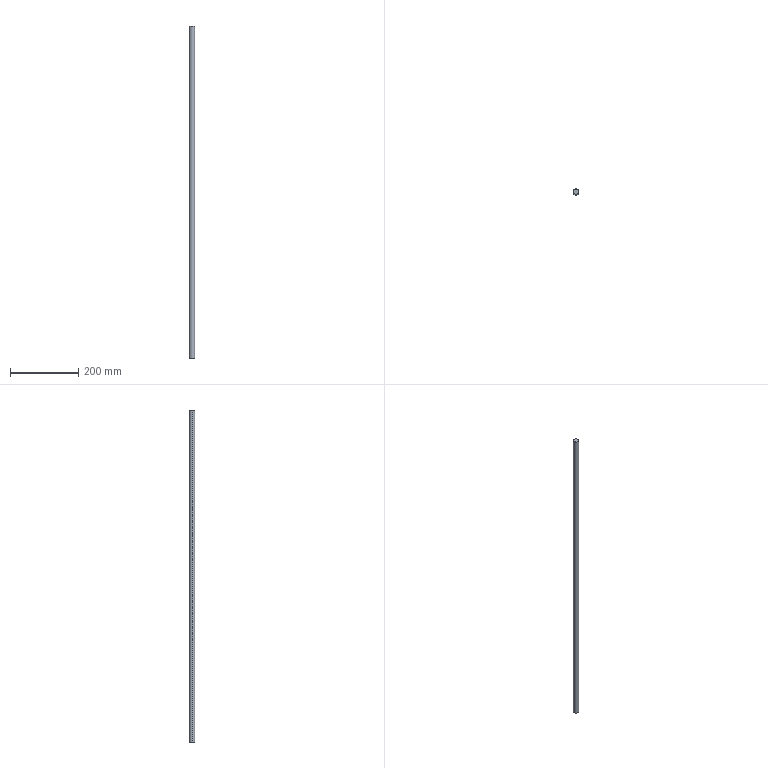Part | SolidWorks | features Extrusion 1 | 1 solid | 4 faces | box 16 x 16 x 970 mm | volume 195030 mm3 | cylinder 2 | plane 2 | commonest cylinder face diameters 16 x2
STEP:
#1=CARTESIAN_POINT('',(8.,0.,-485.));
#2=VERTEX_POINT('',#1);
#3=CARTESIAN_POINT('',(-8.,0.,-485.));
#4=VERTEX_POINT('',#3);
#5=CARTESIAN_POINT('',(0.,0.,-485.));
#6=DIRECTION('',(0.,0.,1.));
#7=DIRECTION('',(1.,0.,0.));
#8=AXIS2_PLACEMENT_3D('',#5,#6,#7);
#9=CIRCLE('',#8,8.);
#10=EDGE_CURVE('',#2,#4,#9,.T.);
#11=ORIENTED_EDGE('',*,*,#10,.T.);
#12=CARTESIAN_POINT('',(-8.,0.,485.));
#13=VERTEX_POINT('',#12);
#14=CARTESIAN_POINT('',(-8.,0.,-485.));
#15=DIRECTION('',(0.,0.,1.));
#16=VECTOR('',#15,1000.);
#17=LINE('',#14,#16);
#18=EDGE_CURVE('',#4,#13,#17,.T.);
#19=ORIENTED_EDGE('',*,*,#18,.T.);
#20=CARTESIAN_POINT('',(8.,0.,485.));
#21=VERTEX_POINT('',#20);
#22=CARTESIAN_POINT('',(0.,0.,485.));
#23=DIRECTION('',(0.,0.,1.));
#24=DIRECTION('',(1.,0.,0.));
#25=AXIS2_PLACEMENT_3D('',#22,#23,#24);
#26=CIRCLE('',#25,8.);
#27=EDGE_CURVE('',#21,#13,#26,.T.);
#28=ORIENTED_EDGE('',*,*,#27,.F.);
#29=CARTESIAN_POINT('',(8.,0.,-485.));
#30=DIRECTION('',(0.,0.,1.));
#31=VECTOR('',#30,1000.);
#32=LINE('',#29,#31);
#33=EDGE_CURVE('',#2,#21,#32,.T.);
#34=ORIENTED_EDGE('',*,*,#33,.F.);
#35=EDGE_LOOP('',(#11,#19,#28,#34));
#36=FACE_OUTER_BOUND('',#35,.T.);
#37=CARTESIAN_POINT('',(0.,0.,-485.));
#38=DIRECTION('',(0.,0.,1.));
#39=DIRECTION('',(1.,0.,0.));
#40=AXIS2_PLACEMENT_3D('',#37,#38,#39);
#41=CYLINDRICAL_SURFACE('',#40,8.);
#42=ADVANCED_FACE('',(#36),#41,.T.);
#43=ORIENTED_EDGE('',*,*,#18,.F.);
#44=CARTESIAN_POINT('',(0.,0.,-485.));
#45=DIRECTION('',(0.,0.,1.));
#46=DIRECTION('',(1.,0.,0.));
#47=AXIS2_PLACEMENT_3D('',#44,#45,#46);
#48=CIRCLE('',#47,8.);
#49=EDGE_CURVE('',#4,#2,#48,.T.);
#50=ORIENTED_EDGE('',*,*,#49,.T.);
#51=ORIENTED_EDGE('',*,*,#33,.T.);
#52=CARTESIAN_POINT('',(0.,0.,485.));
#53=DIRECTION('',(0.,0.,1.));
#54=DIRECTION('',(1.,0.,0.));
#55=AXIS2_PLACEMENT_3D('',#52,#53,#54);
#56=CIRCLE('',#55,8.);
#57=EDGE_CURVE('',#13,#21,#56,.T.);
#58=ORIENTED_EDGE('',*,*,#57,.F.);
#59=EDGE_LOOP('',(#43,#50,#51,#58));
#60=FACE_OUTER_BOUND('',#59,.T.);
#61=CARTESIAN_POINT('',(0.,0.,-485.));
#62=DIRECTION('',(0.,0.,1.));
#63=DIRECTION('',(1.,0.,0.));
#64=AXIS2_PLACEMENT_3D('',#61,#62,#63);
#65=CYLINDRICAL_SURFACE('',#64,8.);
#66=ADVANCED_FACE('',(#60),#65,.T.);
#67=ORIENTED_EDGE('',*,*,#10,.F.);
#68=ORIENTED_EDGE('',*,*,#49,.F.);
#69=EDGE_LOOP('',(#67,#68));
#70=FACE_OUTER_BOUND('',#69,.T.);
#71=CARTESIAN_POINT('',(0.,0.,-485.));
#72=DIRECTION('',(0.,0.,1.));
#73=DIRECTION('',(1.,0.,0.));
#74=AXIS2_PLACEMENT_3D('',#71,#72,#73);
#75=PLANE('',#74);
#76=ADVANCED_FACE('',(#70),#75,.F.);
#77=ORIENTED_EDGE('',*,*,#27,.T.);
#78=ORIENTED_EDGE('',*,*,#57,.T.);
#79=EDGE_LOOP('',(#77,#78));
#80=FACE_OUTER_BOUND('',#79,.T.);
#81=CARTESIAN_POINT('',(0.,0.,485.));
#82=DIRECTION('',(0.,0.,1.));
#83=DIRECTION('',(1.,0.,0.));
#84=AXIS2_PLACEMENT_3D('',#81,#82,#83);
#85=PLANE('',#84);
#86=ADVANCED_FACE('',(#80),#85,.T.);
#87=CLOSED_SHELL('',(#42,#66,#76,#86));
#88=MANIFOLD_SOLID_BREP('',#87);
#89=CARTESIAN_POINT('',(0.,0.,0.));
#90=DIRECTION('',(0.,0.,1.));
#91=DIRECTION('',(1.,0.,0.));
#92=AXIS2_PLACEMENT_3D('',#89,#90,#91);
#93=(LENGTH_UNIT()NAMED_UNIT(*)SI_UNIT(.MILLI.,.METRE.));
#94=UNCERTAINTY_MEASURE_WITH_UNIT(LENGTH_MEASURE(0.00001),#93,'','');
#95=(NAMED_UNIT(*)PLANE_ANGLE_UNIT()SI_UNIT($,.RADIAN.));
#96=(NAMED_UNIT(*)SI_UNIT($,.STERADIAN.)SOLID_ANGLE_UNIT());
#97=(GEOMETRIC_REPRESENTATION_CONTEXT(3)GLOBAL_UNCERTAINTY_ASSIGNED_CONTEXT((#94))GLOBAL_UNIT_ASSIGNED_CONTEXT((#93,#95,#96))REPRESENTATION_CONTEXT('',''));
#98=ADVANCED_BREP_SHAPE_REPRESENTATION('',(#88,#92),#97);